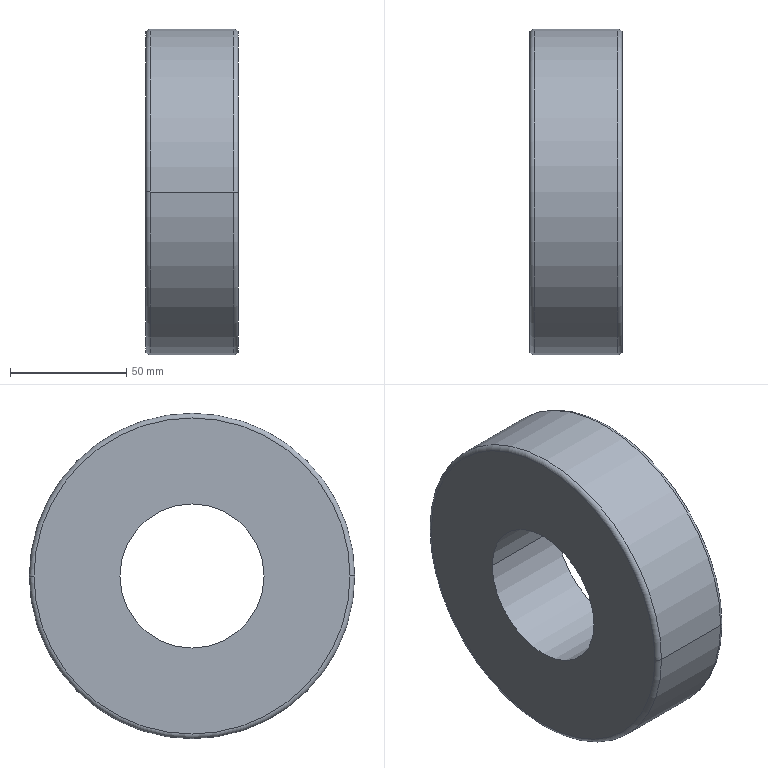Part | SolidWorks | features Fillet 1, ICE 1, Revolution 1 | 1 solid | 10 faces | box 40 x 140 x 140 mm | volume 494239 mm3 | torus 4 | cylinder 4 | plane 2 | commonest cylinder face diameters 62 x2 140 x2
STEP:
#1=CARTESIAN_POINT('',(-20.,-68.,0.));
#2=VERTEX_POINT('',#1);
#3=CARTESIAN_POINT('',(-20.,68.,0.));
#4=VERTEX_POINT('',#3);
#5=CARTESIAN_POINT('',(-20.,0.,0.));
#6=DIRECTION('',(-1.,0.,0.));
#7=DIRECTION('',(0.,1.,0.));
#8=AXIS2_PLACEMENT_3D('',#5,#6,#7);
#9=CIRCLE('',#8,68.);
#10=EDGE_CURVE('',#2,#4,#9,.T.);
#11=ORIENTED_EDGE('',*,*,#10,.F.);
#12=CARTESIAN_POINT('',(-18.,-70.,0.));
#13=VERTEX_POINT('',#12);
#14=CARTESIAN_POINT('',(-18.,-68.,0.));
#15=DIRECTION('',(0.,0.,1.));
#16=DIRECTION('',(0.,-1.,0.));
#17=AXIS2_PLACEMENT_3D('',#14,#15,#16);
#18=CIRCLE('',#17,2.);
#19=EDGE_CURVE('',#2,#13,#18,.T.);
#20=ORIENTED_EDGE('',*,*,#19,.T.);
#21=CARTESIAN_POINT('',(-18.,70.,0.));
#22=VERTEX_POINT('',#21);
#23=CARTESIAN_POINT('',(-18.,0.,0.));
#24=DIRECTION('',(1.,0.,0.));
#25=DIRECTION('',(0.,1.,0.));
#26=AXIS2_PLACEMENT_3D('',#23,#24,#25);
#27=CIRCLE('',#26,70.);
#28=EDGE_CURVE('',#22,#13,#27,.T.);
#29=ORIENTED_EDGE('',*,*,#28,.F.);
#30=CARTESIAN_POINT('',(-18.,68.,0.));
#31=DIRECTION('',(0.,0.,-1.));
#32=DIRECTION('',(-1.,0.,0.));
#33=AXIS2_PLACEMENT_3D('',#30,#31,#32);
#34=CIRCLE('',#33,2.);
#35=EDGE_CURVE('',#4,#22,#34,.T.);
#36=ORIENTED_EDGE('',*,*,#35,.F.);
#37=EDGE_LOOP('',(#11,#20,#29,#36));
#38=FACE_OUTER_BOUND('',#37,.T.);
#39=CARTESIAN_POINT('',(-18.,0.,0.));
#40=DIRECTION('',(1.,0.,0.));
#41=DIRECTION('',(0.,1.,0.));
#42=AXIS2_PLACEMENT_3D('',#39,#40,#41);
#43=TOROIDAL_SURFACE('',#42,68.,2.);
#44=ADVANCED_FACE('',(#38),#43,.T.);
#45=CARTESIAN_POINT('',(20.,68.,0.));
#46=VERTEX_POINT('',#45);
#47=CARTESIAN_POINT('',(20.,-68.,0.));
#48=VERTEX_POINT('',#47);
#49=CARTESIAN_POINT('',(20.,0.,0.));
#50=DIRECTION('',(1.,0.,0.));
#51=DIRECTION('',(0.,-1.,0.));
#52=AXIS2_PLACEMENT_3D('',#49,#50,#51);
#53=CIRCLE('',#52,68.);
#54=EDGE_CURVE('',#46,#48,#53,.T.);
#55=ORIENTED_EDGE('',*,*,#54,.F.);
#56=CARTESIAN_POINT('',(18.,70.,0.));
#57=VERTEX_POINT('',#56);
#58=CARTESIAN_POINT('',(18.,68.,0.));
#59=DIRECTION('',(0.,0.,1.));
#60=DIRECTION('',(0.,-1.,0.));
#61=AXIS2_PLACEMENT_3D('',#58,#59,#60);
#62=CIRCLE('',#61,2.);
#63=EDGE_CURVE('',#46,#57,#62,.T.);
#64=ORIENTED_EDGE('',*,*,#63,.T.);
#65=CARTESIAN_POINT('',(18.,-70.,0.));
#66=VERTEX_POINT('',#65);
#67=CARTESIAN_POINT('',(18.,0.,0.));
#68=DIRECTION('',(-1.,0.,0.));
#69=DIRECTION('',(0.,-1.,0.));
#70=AXIS2_PLACEMENT_3D('',#67,#68,#69);
#71=CIRCLE('',#70,70.);
#72=EDGE_CURVE('',#66,#57,#71,.T.);
#73=ORIENTED_EDGE('',*,*,#72,.F.);
#74=CARTESIAN_POINT('',(18.,-68.,0.));
#75=DIRECTION('',(0.,0.,-1.));
#76=DIRECTION('',(-1.,0.,0.));
#77=AXIS2_PLACEMENT_3D('',#74,#75,#76);
#78=CIRCLE('',#77,2.);
#79=EDGE_CURVE('',#48,#66,#78,.T.);
#80=ORIENTED_EDGE('',*,*,#79,.F.);
#81=EDGE_LOOP('',(#55,#64,#73,#80));
#82=FACE_OUTER_BOUND('',#81,.T.);
#83=CARTESIAN_POINT('',(18.,0.,0.));
#84=DIRECTION('',(-1.,0.,0.));
#85=DIRECTION('',(0.,-1.,0.));
#86=AXIS2_PLACEMENT_3D('',#83,#84,#85);
#87=TOROIDAL_SURFACE('',#86,68.,2.);
#88=ADVANCED_FACE('',(#82),#87,.T.);
#89=CARTESIAN_POINT('',(-20.,-31.,0.));
#90=VERTEX_POINT('',#89);
#91=CARTESIAN_POINT('',(-20.,31.,0.));
#92=VERTEX_POINT('',#91);
#93=CARTESIAN_POINT('',(-20.,0.,0.));
#94=DIRECTION('',(1.,0.,0.));
#95=DIRECTION('',(0.,1.,0.));
#96=AXIS2_PLACEMENT_3D('',#93,#94,#95);
#97=CIRCLE('',#96,31.);
#98=EDGE_CURVE('',#90,#92,#97,.T.);
#99=ORIENTED_EDGE('',*,*,#98,.F.);
#100=CARTESIAN_POINT('',(20.,-31.,0.));
#101=VERTEX_POINT('',#100);
#102=CARTESIAN_POINT('',(-20.,-31.,0.));
#103=DIRECTION('',(1.,0.,0.));
#104=VECTOR('',#103,1000.);
#105=LINE('',#102,#104);
#106=EDGE_CURVE('',#90,#101,#105,.T.);
#107=ORIENTED_EDGE('',*,*,#106,.T.);
#108=CARTESIAN_POINT('',(20.,31.,0.));
#109=VERTEX_POINT('',#108);
#110=CARTESIAN_POINT('',(20.,0.,0.));
#111=DIRECTION('',(1.,0.,0.));
#112=DIRECTION('',(0.,1.,0.));
#113=AXIS2_PLACEMENT_3D('',#110,#111,#112);
#114=CIRCLE('',#113,31.);
#115=EDGE_CURVE('',#101,#109,#114,.T.);
#116=ORIENTED_EDGE('',*,*,#115,.T.);
#117=CARTESIAN_POINT('',(-20.,31.,0.));
#118=DIRECTION('',(1.,0.,0.));
#119=VECTOR('',#118,1000.);
#120=LINE('',#117,#119);
#121=EDGE_CURVE('',#92,#109,#120,.T.);
#122=ORIENTED_EDGE('',*,*,#121,.F.);
#123=EDGE_LOOP('',(#99,#107,#116,#122));
#124=FACE_OUTER_BOUND('',#123,.T.);
#125=CARTESIAN_POINT('',(-20.,0.,0.));
#126=DIRECTION('',(1.,0.,0.));
#127=DIRECTION('',(0.,1.,0.));
#128=AXIS2_PLACEMENT_3D('',#125,#126,#127);
#129=CYLINDRICAL_SURFACE('',#128,31.);
#130=ADVANCED_FACE('',(#124),#129,.F.);
#131=ORIENTED_EDGE('',*,*,#72,.T.);
#132=CARTESIAN_POINT('',(-20.,70.,0.));
#133=DIRECTION('',(-1.,0.,0.));
#134=VECTOR('',#133,1000.);
#135=LINE('',#132,#134);
#136=EDGE_CURVE('',#57,#22,#135,.T.);
#137=ORIENTED_EDGE('',*,*,#136,.T.);
#138=ORIENTED_EDGE('',*,*,#28,.T.);
#139=CARTESIAN_POINT('',(-20.,-70.,0.));
#140=DIRECTION('',(-1.,0.,0.));
#141=VECTOR('',#140,1000.);
#142=LINE('',#139,#141);
#143=EDGE_CURVE('',#66,#13,#142,.T.);
#144=ORIENTED_EDGE('',*,*,#143,.F.);
#145=EDGE_LOOP('',(#131,#137,#138,#144));
#146=FACE_OUTER_BOUND('',#145,.T.);
#147=CARTESIAN_POINT('',(-20.,0.,0.));
#148=DIRECTION('',(-1.,0.,0.));
#149=DIRECTION('',(0.,-1.,0.));
#150=AXIS2_PLACEMENT_3D('',#147,#148,#149);
#151=CYLINDRICAL_SURFACE('',#150,70.);
#152=ADVANCED_FACE('',(#146),#151,.T.);
#153=ORIENTED_EDGE('',*,*,#136,.F.);
#154=CARTESIAN_POINT('',(18.,0.,0.));
#155=DIRECTION('',(-1.,0.,0.));
#156=DIRECTION('',(0.,-1.,0.));
#157=AXIS2_PLACEMENT_3D('',#154,#155,#156);
#158=CIRCLE('',#157,70.);
#159=EDGE_CURVE('',#57,#66,#158,.T.);
#160=ORIENTED_EDGE('',*,*,#159,.T.);
#161=ORIENTED_EDGE('',*,*,#143,.T.);
#162=CARTESIAN_POINT('',(-18.,0.,0.));
#163=DIRECTION('',(1.,0.,0.));
#164=DIRECTION('',(0.,1.,0.));
#165=AXIS2_PLACEMENT_3D('',#162,#163,#164);
#166=CIRCLE('',#165,70.);
#167=EDGE_CURVE('',#13,#22,#166,.T.);
#168=ORIENTED_EDGE('',*,*,#167,.T.);
#169=EDGE_LOOP('',(#153,#160,#161,#168));
#170=FACE_OUTER_BOUND('',#169,.T.);
#171=CARTESIAN_POINT('',(-20.,0.,0.));
#172=DIRECTION('',(-1.,0.,0.));
#173=DIRECTION('',(0.,-1.,0.));
#174=AXIS2_PLACEMENT_3D('',#171,#172,#173);
#175=CYLINDRICAL_SURFACE('',#174,70.);
#176=ADVANCED_FACE('',(#170),#175,.T.);
#177=CARTESIAN_POINT('',(20.,0.,0.));
#178=DIRECTION('',(1.,0.,0.));
#179=DIRECTION('',(0.,-1.,0.));
#180=AXIS2_PLACEMENT_3D('',#177,#178,#179);
#181=CIRCLE('',#180,68.);
#182=EDGE_CURVE('',#48,#46,#181,.T.);
#183=ORIENTED_EDGE('',*,*,#182,.T.);
#184=ORIENTED_EDGE('',*,*,#54,.T.);
#185=EDGE_LOOP('',(#183,#184));
#186=FACE_OUTER_BOUND('',#185,.T.);
#187=CARTESIAN_POINT('',(20.,0.,0.));
#188=DIRECTION('',(1.,0.,0.));
#189=DIRECTION('',(0.,1.,0.));
#190=AXIS2_PLACEMENT_3D('',#187,#188,#189);
#191=CIRCLE('',#190,31.);
#192=EDGE_CURVE('',#109,#101,#191,.T.);
#193=ORIENTED_EDGE('',*,*,#192,.F.);
#194=ORIENTED_EDGE('',*,*,#115,.F.);
#195=EDGE_LOOP('',(#193,#194));
#196=FACE_BOUND('',#195,.T.);
#197=CARTESIAN_POINT('',(20.,70.,0.));
#198=DIRECTION('',(-1.,0.,0.));
#199=DIRECTION('',(0.,-1.,0.));
#200=AXIS2_PLACEMENT_3D('',#197,#198,#199);
#201=PLANE('',#200);
#202=ADVANCED_FACE('',(#186,#196),#201,.F.);
#203=CARTESIAN_POINT('',(-20.,0.,0.));
#204=DIRECTION('',(-1.,0.,0.));
#205=DIRECTION('',(0.,1.,0.));
#206=AXIS2_PLACEMENT_3D('',#203,#204,#205);
#207=CIRCLE('',#206,68.);
#208=EDGE_CURVE('',#4,#2,#207,.T.);
#209=ORIENTED_EDGE('',*,*,#208,.T.);
#210=ORIENTED_EDGE('',*,*,#10,.T.);
#211=EDGE_LOOP('',(#209,#210));
#212=FACE_OUTER_BOUND('',#211,.T.);
#213=CARTESIAN_POINT('',(-20.,0.,0.));
#214=DIRECTION('',(1.,0.,0.));
#215=DIRECTION('',(0.,1.,0.));
#216=AXIS2_PLACEMENT_3D('',#213,#214,#215);
#217=CIRCLE('',#216,31.);
#218=EDGE_CURVE('',#92,#90,#217,.T.);
#219=ORIENTED_EDGE('',*,*,#218,.T.);
#220=ORIENTED_EDGE('',*,*,#98,.T.);
#221=EDGE_LOOP('',(#219,#220));
#222=FACE_BOUND('',#221,.T.);
#223=CARTESIAN_POINT('',(-20.,70.,0.));
#224=DIRECTION('',(1.,0.,0.));
#225=DIRECTION('',(0.,1.,0.));
#226=AXIS2_PLACEMENT_3D('',#223,#224,#225);
#227=PLANE('',#226);
#228=ADVANCED_FACE('',(#212,#222),#227,.F.);
#229=ORIENTED_EDGE('',*,*,#106,.F.);
#230=ORIENTED_EDGE('',*,*,#218,.F.);
#231=ORIENTED_EDGE('',*,*,#121,.T.);
#232=ORIENTED_EDGE('',*,*,#192,.T.);
#233=EDGE_LOOP('',(#229,#230,#231,#232));
#234=FACE_OUTER_BOUND('',#233,.T.);
#235=CARTESIAN_POINT('',(-20.,0.,0.));
#236=DIRECTION('',(1.,0.,0.));
#237=DIRECTION('',(0.,1.,0.));
#238=AXIS2_PLACEMENT_3D('',#235,#236,#237);
#239=CYLINDRICAL_SURFACE('',#238,31.);
#240=ADVANCED_FACE('',(#234),#239,.F.);
#241=ORIENTED_EDGE('',*,*,#63,.F.);
#242=ORIENTED_EDGE('',*,*,#182,.F.);
#243=ORIENTED_EDGE('',*,*,#79,.T.);
#244=ORIENTED_EDGE('',*,*,#159,.F.);
#245=EDGE_LOOP('',(#241,#242,#243,#244));
#246=FACE_OUTER_BOUND('',#245,.T.);
#247=CARTESIAN_POINT('',(18.,0.,0.));
#248=DIRECTION('',(-1.,0.,0.));
#249=DIRECTION('',(0.,-1.,0.));
#250=AXIS2_PLACEMENT_3D('',#247,#248,#249);
#251=TOROIDAL_SURFACE('',#250,68.,2.);
#252=ADVANCED_FACE('',(#246),#251,.T.);
#253=ORIENTED_EDGE('',*,*,#19,.F.);
#254=ORIENTED_EDGE('',*,*,#208,.F.);
#255=ORIENTED_EDGE('',*,*,#35,.T.);
#256=ORIENTED_EDGE('',*,*,#167,.F.);
#257=EDGE_LOOP('',(#253,#254,#255,#256));
#258=FACE_OUTER_BOUND('',#257,.T.);
#259=CARTESIAN_POINT('',(-18.,0.,0.));
#260=DIRECTION('',(1.,0.,0.));
#261=DIRECTION('',(0.,1.,0.));
#262=AXIS2_PLACEMENT_3D('',#259,#260,#261);
#263=TOROIDAL_SURFACE('',#262,68.,2.);
#264=ADVANCED_FACE('',(#258),#263,.T.);
#265=CLOSED_SHELL('',(#44,#88,#130,#152,#176,#202,#228,#240,#252,#264));
#266=MANIFOLD_SOLID_BREP('',#265);
#267=CARTESIAN_POINT('',(0.,0.,0.));
#268=DIRECTION('',(0.,0.,1.));
#269=DIRECTION('',(1.,0.,0.));
#270=AXIS2_PLACEMENT_3D('',#267,#268,#269);
#271=(LENGTH_UNIT()NAMED_UNIT(*)SI_UNIT(.MILLI.,.METRE.));
#272=UNCERTAINTY_MEASURE_WITH_UNIT(LENGTH_MEASURE(0.00001),#271,'','');
#273=(NAMED_UNIT(*)PLANE_ANGLE_UNIT()SI_UNIT($,.RADIAN.));
#274=(NAMED_UNIT(*)SI_UNIT($,.STERADIAN.)SOLID_ANGLE_UNIT());
#275=(GEOMETRIC_REPRESENTATION_CONTEXT(3)GLOBAL_UNCERTAINTY_ASSIGNED_CONTEXT((#272))GLOBAL_UNIT_ASSIGNED_CONTEXT((#271,#273,#274))REPRESENTATION_CONTEXT('',''));
#276=ADVANCED_BREP_SHAPE_REPRESENTATION('',(#266,#270),#275);